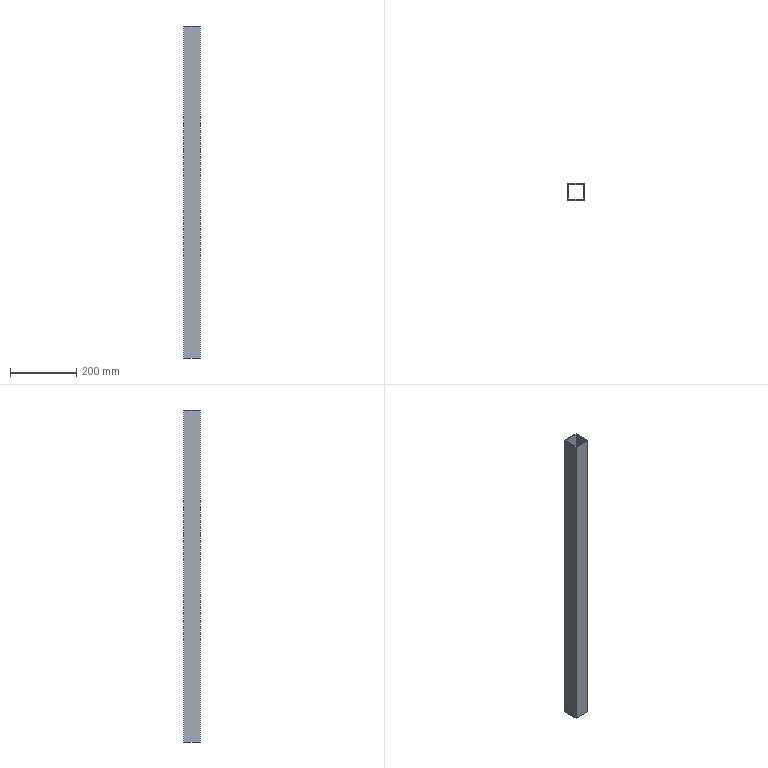Part | STEP file | BCC3 H19_5 | 1 solid | 10 faces | box 50 x 50 x 1000 mm | volume 564000 mm3 | plane 10
STEP:
#1=CARTESIAN_POINT('',(0.,0.,0.));
#2=DIRECTION('',(0.,0.,1.));
#3=DIRECTION('',(1.,0.,0.));
#4=AXIS2_PLACEMENT_3D('',#1,#2,#3);
#5=CARTESIAN_POINT('',(-25.,25.,500.));
#6=VERTEX_POINT('',#5);
#7=CARTESIAN_POINT('',(-25.,-25.,500.));
#8=VERTEX_POINT('',#7);
#9=CARTESIAN_POINT('',(-25.,25.,500.));
#10=DIRECTION('',(0.,-1.,0.));
#11=VECTOR('',#10,1.);
#12=LINE('',#9,#11);
#13=CARTESIAN_POINT('',(0.,0.,500.));
#14=DIRECTION('',(0.,0.,1.));
#15=DIRECTION('',(1.,0.,0.));
#16=AXIS2_PLACEMENT_3D('',#13,#14,#15);
#17=PLANE('',#16);
#18=CARTESIAN_POINT('',(-25.,25.));
#19=DIRECTION('',(0.,-1.));
#20=VECTOR('',#19,1.);
#21=LINE('',#18,#20);
#22=(GEOMETRIC_REPRESENTATION_CONTEXT(2)PARAMETRIC_REPRESENTATION_CONTEXT()REPRESENTATION_CONTEXT('',''));
#23=DEFINITIONAL_REPRESENTATION('',(#21),#22);
#24=PCURVE('',#17,#23);
#25=CARTESIAN_POINT('',(-25.,25.,500.));
#26=DIRECTION('',(1.,0.,0.));
#27=DIRECTION('',(0.,1.,0.));
#28=AXIS2_PLACEMENT_3D('',#25,#26,#27);
#29=PLANE('',#28);
#30=CARTESIAN_POINT('',(0.,0.));
#31=DIRECTION('',(-1.,0.));
#32=VECTOR('',#31,1.);
#33=LINE('',#30,#32);
#34=(GEOMETRIC_REPRESENTATION_CONTEXT(2)PARAMETRIC_REPRESENTATION_CONTEXT()REPRESENTATION_CONTEXT('',''));
#35=DEFINITIONAL_REPRESENTATION('',(#33),#34);
#36=PCURVE('',#29,#35);
#37=SURFACE_CURVE('',#12,(#24,#36),.PCURVE_S1.);
#38=EDGE_CURVE('',#6,#8,#37,.T.);
#39=ORIENTED_EDGE('',*,*,#38,.T.);
#40=CARTESIAN_POINT('',(25.,-25.,500.));
#41=VERTEX_POINT('',#40);
#42=CARTESIAN_POINT('',(-25.,-25.,500.));
#43=DIRECTION('',(1.,0.,0.));
#44=VECTOR('',#43,1.);
#45=LINE('',#42,#44);
#46=CARTESIAN_POINT('',(-25.,-25.));
#47=DIRECTION('',(1.,0.));
#48=VECTOR('',#47,1.);
#49=LINE('',#46,#48);
#50=(GEOMETRIC_REPRESENTATION_CONTEXT(2)PARAMETRIC_REPRESENTATION_CONTEXT()REPRESENTATION_CONTEXT('',''));
#51=DEFINITIONAL_REPRESENTATION('',(#49),#50);
#52=PCURVE('',#17,#51);
#53=CARTESIAN_POINT('',(-25.,-25.,500.));
#54=DIRECTION('',(0.,1.,0.));
#55=DIRECTION('',(0.,0.,1.));
#56=AXIS2_PLACEMENT_3D('',#53,#54,#55);
#57=PLANE('',#56);
#58=CARTESIAN_POINT('',(0.,0.));
#59=DIRECTION('',(0.,1.));
#60=VECTOR('',#59,1.);
#61=LINE('',#58,#60);
#62=(GEOMETRIC_REPRESENTATION_CONTEXT(2)PARAMETRIC_REPRESENTATION_CONTEXT()REPRESENTATION_CONTEXT('',''));
#63=DEFINITIONAL_REPRESENTATION('',(#61),#62);
#64=PCURVE('',#57,#63);
#65=SURFACE_CURVE('',#45,(#52,#64),.PCURVE_S1.);
#66=EDGE_CURVE('',#8,#41,#65,.T.);
#67=ORIENTED_EDGE('',*,*,#66,.T.);
#68=CARTESIAN_POINT('',(25.,25.,500.));
#69=VERTEX_POINT('',#68);
#70=CARTESIAN_POINT('',(25.,25.,500.));
#71=DIRECTION('',(0.,1.,0.));
#72=VECTOR('',#71,1.);
#73=LINE('',#70,#72);
#74=CARTESIAN_POINT('',(25.,25.));
#75=DIRECTION('',(0.,1.));
#76=VECTOR('',#75,1.);
#77=LINE('',#74,#76);
#78=(GEOMETRIC_REPRESENTATION_CONTEXT(2)PARAMETRIC_REPRESENTATION_CONTEXT()REPRESENTATION_CONTEXT('',''));
#79=DEFINITIONAL_REPRESENTATION('',(#77),#78);
#80=PCURVE('',#17,#79);
#81=CARTESIAN_POINT('',(25.,25.,500.));
#82=DIRECTION('',(-1.,0.,0.));
#83=DIRECTION('',(0.,-1.,0.));
#84=AXIS2_PLACEMENT_3D('',#81,#82,#83);
#85=PLANE('',#84);
#86=CARTESIAN_POINT('',(0.,0.));
#87=DIRECTION('',(-1.,0.));
#88=VECTOR('',#87,1.);
#89=LINE('',#86,#88);
#90=(GEOMETRIC_REPRESENTATION_CONTEXT(2)PARAMETRIC_REPRESENTATION_CONTEXT()REPRESENTATION_CONTEXT('',''));
#91=DEFINITIONAL_REPRESENTATION('',(#89),#90);
#92=PCURVE('',#85,#91);
#93=SURFACE_CURVE('',#73,(#80,#92),.PCURVE_S1.);
#94=EDGE_CURVE('',#41,#69,#93,.T.);
#95=ORIENTED_EDGE('',*,*,#94,.T.);
#96=CARTESIAN_POINT('',(-25.,25.,500.));
#97=DIRECTION('',(-1.,0.,0.));
#98=VECTOR('',#97,1.);
#99=LINE('',#96,#98);
#100=CARTESIAN_POINT('',(-25.,25.));
#101=DIRECTION('',(-1.,0.));
#102=VECTOR('',#101,1.);
#103=LINE('',#100,#102);
#104=(GEOMETRIC_REPRESENTATION_CONTEXT(2)PARAMETRIC_REPRESENTATION_CONTEXT()REPRESENTATION_CONTEXT('',''));
#105=DEFINITIONAL_REPRESENTATION('',(#103),#104);
#106=PCURVE('',#17,#105);
#107=CARTESIAN_POINT('',(-25.,25.,500.));
#108=DIRECTION('',(0.,-1.,0.));
#109=DIRECTION('',(0.,0.,-1.));
#110=AXIS2_PLACEMENT_3D('',#107,#108,#109);
#111=PLANE('',#110);
#112=CARTESIAN_POINT('',(0.,0.));
#113=DIRECTION('',(0.,-1.));
#114=VECTOR('',#113,1.);
#115=LINE('',#112,#114);
#116=(GEOMETRIC_REPRESENTATION_CONTEXT(2)PARAMETRIC_REPRESENTATION_CONTEXT()REPRESENTATION_CONTEXT('',''));
#117=DEFINITIONAL_REPRESENTATION('',(#115),#116);
#118=PCURVE('',#111,#117);
#119=SURFACE_CURVE('',#99,(#106,#118),.PCURVE_S1.);
#120=EDGE_CURVE('',#69,#6,#119,.T.);
#121=ORIENTED_EDGE('',*,*,#120,.T.);
#122=EDGE_LOOP('',(#39,#67,#95,#121));
#123=FACE_BOUND('',#122,.T.);
#124=CARTESIAN_POINT('',(-22.,-22.,500.));
#125=VERTEX_POINT('',#124);
#126=CARTESIAN_POINT('',(22.,-22.,500.));
#127=VERTEX_POINT('',#126);
#128=CARTESIAN_POINT('',(-22.,-22.,500.));
#129=DIRECTION('',(1.,0.,0.));
#130=VECTOR('',#129,1.);
#131=LINE('',#128,#130);
#132=CARTESIAN_POINT('',(-22.,-22.));
#133=DIRECTION('',(1.,0.));
#134=VECTOR('',#133,1.);
#135=LINE('',#132,#134);
#136=(GEOMETRIC_REPRESENTATION_CONTEXT(2)PARAMETRIC_REPRESENTATION_CONTEXT()REPRESENTATION_CONTEXT('',''));
#137=DEFINITIONAL_REPRESENTATION('',(#135),#136);
#138=PCURVE('',#17,#137);
#139=CARTESIAN_POINT('',(-22.,-22.,500.));
#140=DIRECTION('',(0.,1.,0.));
#141=DIRECTION('',(-1.,0.,0.));
#142=AXIS2_PLACEMENT_3D('',#139,#140,#141);
#143=PLANE('',#142);
#144=CARTESIAN_POINT('',(0.,0.));
#145=DIRECTION('',(-1.,0.));
#146=VECTOR('',#145,1.);
#147=LINE('',#144,#146);
#148=(GEOMETRIC_REPRESENTATION_CONTEXT(2)PARAMETRIC_REPRESENTATION_CONTEXT()REPRESENTATION_CONTEXT('',''));
#149=DEFINITIONAL_REPRESENTATION('',(#147),#148);
#150=PCURVE('',#143,#149);
#151=SURFACE_CURVE('',#131,(#138,#150),.PCURVE_S1.);
#152=EDGE_CURVE('',#125,#127,#151,.T.);
#153=ORIENTED_EDGE('',*,*,#152,.F.);
#154=CARTESIAN_POINT('',(-22.,22.,500.));
#155=VERTEX_POINT('',#154);
#156=CARTESIAN_POINT('',(-22.,22.,500.));
#157=DIRECTION('',(0.,-1.,0.));
#158=VECTOR('',#157,1.);
#159=LINE('',#156,#158);
#160=CARTESIAN_POINT('',(-22.,22.));
#161=DIRECTION('',(0.,-1.));
#162=VECTOR('',#161,1.);
#163=LINE('',#160,#162);
#164=(GEOMETRIC_REPRESENTATION_CONTEXT(2)PARAMETRIC_REPRESENTATION_CONTEXT()REPRESENTATION_CONTEXT('',''));
#165=DEFINITIONAL_REPRESENTATION('',(#163),#164);
#166=PCURVE('',#17,#165);
#167=CARTESIAN_POINT('',(-22.,22.,500.));
#168=DIRECTION('',(1.,0.,0.));
#169=DIRECTION('',(0.,1.,0.));
#170=AXIS2_PLACEMENT_3D('',#167,#168,#169);
#171=PLANE('',#170);
#172=CARTESIAN_POINT('',(0.,0.));
#173=DIRECTION('',(-1.,0.));
#174=VECTOR('',#173,1.);
#175=LINE('',#172,#174);
#176=(GEOMETRIC_REPRESENTATION_CONTEXT(2)PARAMETRIC_REPRESENTATION_CONTEXT()REPRESENTATION_CONTEXT('',''));
#177=DEFINITIONAL_REPRESENTATION('',(#175),#176);
#178=PCURVE('',#171,#177);
#179=SURFACE_CURVE('',#159,(#166,#178),.PCURVE_S1.);
#180=EDGE_CURVE('',#155,#125,#179,.T.);
#181=ORIENTED_EDGE('',*,*,#180,.F.);
#182=CARTESIAN_POINT('',(22.,22.,500.));
#183=VERTEX_POINT('',#182);
#184=CARTESIAN_POINT('',(-22.,22.,500.));
#185=DIRECTION('',(-1.,0.,0.));
#186=VECTOR('',#185,1.);
#187=LINE('',#184,#186);
#188=CARTESIAN_POINT('',(-22.,22.));
#189=DIRECTION('',(-1.,0.));
#190=VECTOR('',#189,1.);
#191=LINE('',#188,#190);
#192=(GEOMETRIC_REPRESENTATION_CONTEXT(2)PARAMETRIC_REPRESENTATION_CONTEXT()REPRESENTATION_CONTEXT('',''));
#193=DEFINITIONAL_REPRESENTATION('',(#191),#192);
#194=PCURVE('',#17,#193);
#195=CARTESIAN_POINT('',(-22.,22.,500.));
#196=DIRECTION('',(0.,-1.,0.));
#197=DIRECTION('',(0.,0.,-1.));
#198=AXIS2_PLACEMENT_3D('',#195,#196,#197);
#199=PLANE('',#198);
#200=CARTESIAN_POINT('',(0.,0.));
#201=DIRECTION('',(0.,-1.));
#202=VECTOR('',#201,1.);
#203=LINE('',#200,#202);
#204=(GEOMETRIC_REPRESENTATION_CONTEXT(2)PARAMETRIC_REPRESENTATION_CONTEXT()REPRESENTATION_CONTEXT('',''));
#205=DEFINITIONAL_REPRESENTATION('',(#203),#204);
#206=PCURVE('',#199,#205);
#207=SURFACE_CURVE('',#187,(#194,#206),.PCURVE_S1.);
#208=EDGE_CURVE('',#183,#155,#207,.T.);
#209=ORIENTED_EDGE('',*,*,#208,.F.);
#210=CARTESIAN_POINT('',(22.,22.,500.));
#211=DIRECTION('',(0.,1.,0.));
#212=VECTOR('',#211,1.);
#213=LINE('',#210,#212);
#214=CARTESIAN_POINT('',(22.,22.));
#215=DIRECTION('',(0.,1.));
#216=VECTOR('',#215,1.);
#217=LINE('',#214,#216);
#218=(GEOMETRIC_REPRESENTATION_CONTEXT(2)PARAMETRIC_REPRESENTATION_CONTEXT()REPRESENTATION_CONTEXT('',''));
#219=DEFINITIONAL_REPRESENTATION('',(#217),#218);
#220=PCURVE('',#17,#219);
#221=CARTESIAN_POINT('',(22.,22.,500.));
#222=DIRECTION('',(-1.,0.,0.));
#223=DIRECTION('',(0.,-1.,0.));
#224=AXIS2_PLACEMENT_3D('',#221,#222,#223);
#225=PLANE('',#224);
#226=CARTESIAN_POINT('',(0.,0.));
#227=DIRECTION('',(-1.,0.));
#228=VECTOR('',#227,1.);
#229=LINE('',#226,#228);
#230=(GEOMETRIC_REPRESENTATION_CONTEXT(2)PARAMETRIC_REPRESENTATION_CONTEXT()REPRESENTATION_CONTEXT('',''));
#231=DEFINITIONAL_REPRESENTATION('',(#229),#230);
#232=PCURVE('',#225,#231);
#233=SURFACE_CURVE('',#213,(#220,#232),.PCURVE_S1.);
#234=EDGE_CURVE('',#127,#183,#233,.T.);
#235=ORIENTED_EDGE('',*,*,#234,.F.);
#236=EDGE_LOOP('',(#153,#181,#209,#235));
#237=FACE_BOUND('',#236,.T.);
#238=ADVANCED_FACE('',(#123,#237),#17,.T.);
#239=CARTESIAN_POINT('',(-25.,25.,-500.));
#240=VERTEX_POINT('',#239);
#241=CARTESIAN_POINT('',(-25.,-25.,-500.));
#242=VERTEX_POINT('',#241);
#243=CARTESIAN_POINT('',(-25.,25.,-500.));
#244=DIRECTION('',(0.,-1.,0.));
#245=VECTOR('',#244,1.);
#246=LINE('',#243,#245);
#247=CARTESIAN_POINT('',(0.,0.,-500.));
#248=DIRECTION('',(0.,0.,1.));
#249=DIRECTION('',(1.,0.,0.));
#250=AXIS2_PLACEMENT_3D('',#247,#248,#249);
#251=PLANE('',#250);
#252=CARTESIAN_POINT('',(-25.,25.));
#253=DIRECTION('',(0.,-1.));
#254=VECTOR('',#253,1.);
#255=LINE('',#252,#254);
#256=(GEOMETRIC_REPRESENTATION_CONTEXT(2)PARAMETRIC_REPRESENTATION_CONTEXT()REPRESENTATION_CONTEXT('',''));
#257=DEFINITIONAL_REPRESENTATION('',(#255),#256);
#258=PCURVE('',#251,#257);
#259=CARTESIAN_POINT('',(0.,-1000.));
#260=DIRECTION('',(-1.,0.));
#261=VECTOR('',#260,1.);
#262=LINE('',#259,#261);
#263=(GEOMETRIC_REPRESENTATION_CONTEXT(2)PARAMETRIC_REPRESENTATION_CONTEXT()REPRESENTATION_CONTEXT('',''));
#264=DEFINITIONAL_REPRESENTATION('',(#262),#263);
#265=PCURVE('',#29,#264);
#266=SURFACE_CURVE('',#246,(#258,#265),.PCURVE_S1.);
#267=EDGE_CURVE('',#240,#242,#266,.T.);
#268=ORIENTED_EDGE('',*,*,#267,.F.);
#269=CARTESIAN_POINT('',(25.,25.,-500.));
#270=VERTEX_POINT('',#269);
#271=CARTESIAN_POINT('',(-25.,25.,-500.));
#272=DIRECTION('',(-1.,0.,0.));
#273=VECTOR('',#272,1.);
#274=LINE('',#271,#273);
#275=CARTESIAN_POINT('',(-25.,25.));
#276=DIRECTION('',(-1.,0.));
#277=VECTOR('',#276,1.);
#278=LINE('',#275,#277);
#279=(GEOMETRIC_REPRESENTATION_CONTEXT(2)PARAMETRIC_REPRESENTATION_CONTEXT()REPRESENTATION_CONTEXT('',''));
#280=DEFINITIONAL_REPRESENTATION('',(#278),#279);
#281=PCURVE('',#251,#280);
#282=CARTESIAN_POINT('',(1000.,0.));
#283=DIRECTION('',(0.,-1.));
#284=VECTOR('',#283,1.);
#285=LINE('',#282,#284);
#286=(GEOMETRIC_REPRESENTATION_CONTEXT(2)PARAMETRIC_REPRESENTATION_CONTEXT()REPRESENTATION_CONTEXT('',''));
#287=DEFINITIONAL_REPRESENTATION('',(#285),#286);
#288=PCURVE('',#111,#287);
#289=SURFACE_CURVE('',#274,(#281,#288),.PCURVE_S1.);
#290=EDGE_CURVE('',#270,#240,#289,.T.);
#291=ORIENTED_EDGE('',*,*,#290,.F.);
#292=CARTESIAN_POINT('',(25.,-25.,-500.));
#293=VERTEX_POINT('',#292);
#294=CARTESIAN_POINT('',(25.,25.,-500.));
#295=DIRECTION('',(0.,1.,0.));
#296=VECTOR('',#295,1.);
#297=LINE('',#294,#296);
#298=CARTESIAN_POINT('',(25.,25.));
#299=DIRECTION('',(0.,1.));
#300=VECTOR('',#299,1.);
#301=LINE('',#298,#300);
#302=(GEOMETRIC_REPRESENTATION_CONTEXT(2)PARAMETRIC_REPRESENTATION_CONTEXT()REPRESENTATION_CONTEXT('',''));
#303=DEFINITIONAL_REPRESENTATION('',(#301),#302);
#304=PCURVE('',#251,#303);
#305=CARTESIAN_POINT('',(0.,-1000.));
#306=DIRECTION('',(-1.,0.));
#307=VECTOR('',#306,1.);
#308=LINE('',#305,#307);
#309=(GEOMETRIC_REPRESENTATION_CONTEXT(2)PARAMETRIC_REPRESENTATION_CONTEXT()REPRESENTATION_CONTEXT('',''));
#310=DEFINITIONAL_REPRESENTATION('',(#308),#309);
#311=PCURVE('',#85,#310);
#312=SURFACE_CURVE('',#297,(#304,#311),.PCURVE_S1.);
#313=EDGE_CURVE('',#293,#270,#312,.T.);
#314=ORIENTED_EDGE('',*,*,#313,.F.);
#315=CARTESIAN_POINT('',(-25.,-25.,-500.));
#316=DIRECTION('',(1.,0.,0.));
#317=VECTOR('',#316,1.);
#318=LINE('',#315,#317);
#319=CARTESIAN_POINT('',(-25.,-25.));
#320=DIRECTION('',(1.,0.));
#321=VECTOR('',#320,1.);
#322=LINE('',#319,#321);
#323=(GEOMETRIC_REPRESENTATION_CONTEXT(2)PARAMETRIC_REPRESENTATION_CONTEXT()REPRESENTATION_CONTEXT('',''));
#324=DEFINITIONAL_REPRESENTATION('',(#322),#323);
#325=PCURVE('',#251,#324);
#326=CARTESIAN_POINT('',(-1000.,0.));
#327=DIRECTION('',(0.,1.));
#328=VECTOR('',#327,1.);
#329=LINE('',#326,#328);
#330=(GEOMETRIC_REPRESENTATION_CONTEXT(2)PARAMETRIC_REPRESENTATION_CONTEXT()REPRESENTATION_CONTEXT('',''));
#331=DEFINITIONAL_REPRESENTATION('',(#329),#330);
#332=PCURVE('',#57,#331);
#333=SURFACE_CURVE('',#318,(#325,#332),.PCURVE_S1.);
#334=EDGE_CURVE('',#242,#293,#333,.T.);
#335=ORIENTED_EDGE('',*,*,#334,.F.);
#336=EDGE_LOOP('',(#268,#291,#314,#335));
#337=FACE_BOUND('',#336,.T.);
#338=CARTESIAN_POINT('',(-22.,22.,-500.));
#339=VERTEX_POINT('',#338);
#340=CARTESIAN_POINT('',(-22.,-22.,-500.));
#341=VERTEX_POINT('',#340);
#342=CARTESIAN_POINT('',(-22.,22.,-500.));
#343=DIRECTION('',(0.,-1.,0.));
#344=VECTOR('',#343,1.);
#345=LINE('',#342,#344);
#346=CARTESIAN_POINT('',(-22.,22.));
#347=DIRECTION('',(0.,-1.));
#348=VECTOR('',#347,1.);
#349=LINE('',#346,#348);
#350=(GEOMETRIC_REPRESENTATION_CONTEXT(2)PARAMETRIC_REPRESENTATION_CONTEXT()REPRESENTATION_CONTEXT('',''));
#351=DEFINITIONAL_REPRESENTATION('',(#349),#350);
#352=PCURVE('',#251,#351);
#353=CARTESIAN_POINT('',(0.,-1000.));
#354=DIRECTION('',(-1.,0.));
#355=VECTOR('',#354,1.);
#356=LINE('',#353,#355);
#357=(GEOMETRIC_REPRESENTATION_CONTEXT(2)PARAMETRIC_REPRESENTATION_CONTEXT()REPRESENTATION_CONTEXT('',''));
#358=DEFINITIONAL_REPRESENTATION('',(#356),#357);
#359=PCURVE('',#171,#358);
#360=SURFACE_CURVE('',#345,(#352,#359),.PCURVE_S1.);
#361=EDGE_CURVE('',#339,#341,#360,.T.);
#362=ORIENTED_EDGE('',*,*,#361,.T.);
#363=CARTESIAN_POINT('',(22.,-22.,-500.));
#364=VERTEX_POINT('',#363);
#365=CARTESIAN_POINT('',(-22.,-22.,-500.));
#366=DIRECTION('',(1.,0.,0.));
#367=VECTOR('',#366,1.);
#368=LINE('',#365,#367);
#369=CARTESIAN_POINT('',(-22.,-22.));
#370=DIRECTION('',(1.,0.));
#371=VECTOR('',#370,1.);
#372=LINE('',#369,#371);
#373=(GEOMETRIC_REPRESENTATION_CONTEXT(2)PARAMETRIC_REPRESENTATION_CONTEXT()REPRESENTATION_CONTEXT('',''));
#374=DEFINITIONAL_REPRESENTATION('',(#372),#373);
#375=PCURVE('',#251,#374);
#376=CARTESIAN_POINT('',(0.,-1000.));
#377=DIRECTION('',(-1.,0.));
#378=VECTOR('',#377,1.);
#379=LINE('',#376,#378);
#380=(GEOMETRIC_REPRESENTATION_CONTEXT(2)PARAMETRIC_REPRESENTATION_CONTEXT()REPRESENTATION_CONTEXT('',''));
#381=DEFINITIONAL_REPRESENTATION('',(#379),#380);
#382=PCURVE('',#143,#381);
#383=SURFACE_CURVE('',#368,(#375,#382),.PCURVE_S1.);
#384=EDGE_CURVE('',#341,#364,#383,.T.);
#385=ORIENTED_EDGE('',*,*,#384,.T.);
#386=CARTESIAN_POINT('',(22.,22.,-500.));
#387=VERTEX_POINT('',#386);
#388=CARTESIAN_POINT('',(22.,22.,-500.));
#389=DIRECTION('',(0.,1.,0.));
#390=VECTOR('',#389,1.);
#391=LINE('',#388,#390);
#392=CARTESIAN_POINT('',(22.,22.));
#393=DIRECTION('',(0.,1.));
#394=VECTOR('',#393,1.);
#395=LINE('',#392,#394);
#396=(GEOMETRIC_REPRESENTATION_CONTEXT(2)PARAMETRIC_REPRESENTATION_CONTEXT()REPRESENTATION_CONTEXT('',''));
#397=DEFINITIONAL_REPRESENTATION('',(#395),#396);
#398=PCURVE('',#251,#397);
#399=CARTESIAN_POINT('',(0.,-1000.));
#400=DIRECTION('',(-1.,0.));
#401=VECTOR('',#400,1.);
#402=LINE('',#399,#401);
#403=(GEOMETRIC_REPRESENTATION_CONTEXT(2)PARAMETRIC_REPRESENTATION_CONTEXT()REPRESENTATION_CONTEXT('',''));
#404=DEFINITIONAL_REPRESENTATION('',(#402),#403);
#405=PCURVE('',#225,#404);
#406=SURFACE_CURVE('',#391,(#398,#405),.PCURVE_S1.);
#407=EDGE_CURVE('',#364,#387,#406,.T.);
#408=ORIENTED_EDGE('',*,*,#407,.T.);
#409=CARTESIAN_POINT('',(-22.,22.,-500.));
#410=DIRECTION('',(-1.,0.,0.));
#411=VECTOR('',#410,1.);
#412=LINE('',#409,#411);
#413=CARTESIAN_POINT('',(-22.,22.));
#414=DIRECTION('',(-1.,0.));
#415=VECTOR('',#414,1.);
#416=LINE('',#413,#415);
#417=(GEOMETRIC_REPRESENTATION_CONTEXT(2)PARAMETRIC_REPRESENTATION_CONTEXT()REPRESENTATION_CONTEXT('',''));
#418=DEFINITIONAL_REPRESENTATION('',(#416),#417);
#419=PCURVE('',#251,#418);
#420=CARTESIAN_POINT('',(1000.,0.));
#421=DIRECTION('',(0.,-1.));
#422=VECTOR('',#421,1.);
#423=LINE('',#420,#422);
#424=(GEOMETRIC_REPRESENTATION_CONTEXT(2)PARAMETRIC_REPRESENTATION_CONTEXT()REPRESENTATION_CONTEXT('',''));
#425=DEFINITIONAL_REPRESENTATION('',(#423),#424);
#426=PCURVE('',#199,#425);
#427=SURFACE_CURVE('',#412,(#419,#426),.PCURVE_S1.);
#428=EDGE_CURVE('',#387,#339,#427,.T.);
#429=ORIENTED_EDGE('',*,*,#428,.T.);
#430=EDGE_LOOP('',(#362,#385,#408,#429));
#431=FACE_BOUND('',#430,.T.);
#432=ADVANCED_FACE('',(#337,#431),#251,.F.);
#433=ORIENTED_EDGE('',*,*,#267,.T.);
#434=CARTESIAN_POINT('',(-25.,-25.,500.));
#435=DIRECTION('',(0.,0.,-1.));
#436=VECTOR('',#435,1.);
#437=LINE('',#434,#436);
#438=CARTESIAN_POINT('',(-50.,0.));
#439=DIRECTION('',(0.,-1.));
#440=VECTOR('',#439,1.);
#441=LINE('',#438,#440);
#442=(GEOMETRIC_REPRESENTATION_CONTEXT(2)PARAMETRIC_REPRESENTATION_CONTEXT()REPRESENTATION_CONTEXT('',''));
#443=DEFINITIONAL_REPRESENTATION('',(#441),#442);
#444=PCURVE('',#29,#443);
#445=CARTESIAN_POINT('',(0.,0.));
#446=DIRECTION('',(-1.,0.));
#447=VECTOR('',#446,1.);
#448=LINE('',#445,#447);
#449=(GEOMETRIC_REPRESENTATION_CONTEXT(2)PARAMETRIC_REPRESENTATION_CONTEXT()REPRESENTATION_CONTEXT('',''));
#450=DEFINITIONAL_REPRESENTATION('',(#448),#449);
#451=PCURVE('',#57,#450);
#452=SURFACE_CURVE('',#437,(#444,#451),.PCURVE_S1.);
#453=EDGE_CURVE('',#8,#242,#452,.T.);
#454=ORIENTED_EDGE('',*,*,#453,.F.);
#455=ORIENTED_EDGE('',*,*,#38,.F.);
#456=CARTESIAN_POINT('',(-25.,25.,500.));
#457=DIRECTION('',(0.,0.,-1.));
#458=VECTOR('',#457,1.);
#459=LINE('',#456,#458);
#460=CARTESIAN_POINT('',(0.,0.));
#461=DIRECTION('',(0.,-1.));
#462=VECTOR('',#461,1.);
#463=LINE('',#460,#462);
#464=(GEOMETRIC_REPRESENTATION_CONTEXT(2)PARAMETRIC_REPRESENTATION_CONTEXT()REPRESENTATION_CONTEXT('',''));
#465=DEFINITIONAL_REPRESENTATION('',(#463),#464);
#466=PCURVE('',#29,#465);
#467=CARTESIAN_POINT('',(0.,0.));
#468=DIRECTION('',(1.,0.));
#469=VECTOR('',#468,1.);
#470=LINE('',#467,#469);
#471=(GEOMETRIC_REPRESENTATION_CONTEXT(2)PARAMETRIC_REPRESENTATION_CONTEXT()REPRESENTATION_CONTEXT('',''));
#472=DEFINITIONAL_REPRESENTATION('',(#470),#471);
#473=PCURVE('',#111,#472);
#474=SURFACE_CURVE('',#459,(#466,#473),.PCURVE_S1.);
#475=EDGE_CURVE('',#6,#240,#474,.T.);
#476=ORIENTED_EDGE('',*,*,#475,.T.);
#477=EDGE_LOOP('',(#433,#454,#455,#476));
#478=FACE_BOUND('',#477,.T.);
#479=ADVANCED_FACE('',(#478),#29,.F.);
#480=ORIENTED_EDGE('',*,*,#334,.T.);
#481=CARTESIAN_POINT('',(25.,-25.,500.));
#482=DIRECTION('',(0.,0.,-1.));
#483=VECTOR('',#482,1.);
#484=LINE('',#481,#483);
#485=CARTESIAN_POINT('',(0.,50.));
#486=DIRECTION('',(-1.,0.));
#487=VECTOR('',#486,1.);
#488=LINE('',#485,#487);
#489=(GEOMETRIC_REPRESENTATION_CONTEXT(2)PARAMETRIC_REPRESENTATION_CONTEXT()REPRESENTATION_CONTEXT('',''));
#490=DEFINITIONAL_REPRESENTATION('',(#488),#489);
#491=PCURVE('',#57,#490);
#492=CARTESIAN_POINT('',(50.,0.));
#493=DIRECTION('',(0.,-1.));
#494=VECTOR('',#493,1.);
#495=LINE('',#492,#494);
#496=(GEOMETRIC_REPRESENTATION_CONTEXT(2)PARAMETRIC_REPRESENTATION_CONTEXT()REPRESENTATION_CONTEXT('',''));
#497=DEFINITIONAL_REPRESENTATION('',(#495),#496);
#498=PCURVE('',#85,#497);
#499=SURFACE_CURVE('',#484,(#491,#498),.PCURVE_S1.);
#500=EDGE_CURVE('',#41,#293,#499,.T.);
#501=ORIENTED_EDGE('',*,*,#500,.F.);
#502=ORIENTED_EDGE('',*,*,#66,.F.);
#503=ORIENTED_EDGE('',*,*,#453,.T.);
#504=EDGE_LOOP('',(#480,#501,#502,#503));
#505=FACE_BOUND('',#504,.T.);
#506=ADVANCED_FACE('',(#505),#57,.F.);
#507=ORIENTED_EDGE('',*,*,#313,.T.);
#508=CARTESIAN_POINT('',(25.,25.,500.));
#509=DIRECTION('',(0.,0.,-1.));
#510=VECTOR('',#509,1.);
#511=LINE('',#508,#510);
#512=CARTESIAN_POINT('',(0.,0.));
#513=DIRECTION('',(0.,-1.));
#514=VECTOR('',#513,1.);
#515=LINE('',#512,#514);
#516=(GEOMETRIC_REPRESENTATION_CONTEXT(2)PARAMETRIC_REPRESENTATION_CONTEXT()REPRESENTATION_CONTEXT('',''));
#517=DEFINITIONAL_REPRESENTATION('',(#515),#516);
#518=PCURVE('',#85,#517);
#519=CARTESIAN_POINT('',(0.,50.));
#520=DIRECTION('',(1.,0.));
#521=VECTOR('',#520,1.);
#522=LINE('',#519,#521);
#523=(GEOMETRIC_REPRESENTATION_CONTEXT(2)PARAMETRIC_REPRESENTATION_CONTEXT()REPRESENTATION_CONTEXT('',''));
#524=DEFINITIONAL_REPRESENTATION('',(#522),#523);
#525=PCURVE('',#111,#524);
#526=SURFACE_CURVE('',#511,(#518,#525),.PCURVE_S1.);
#527=EDGE_CURVE('',#69,#270,#526,.T.);
#528=ORIENTED_EDGE('',*,*,#527,.F.);
#529=ORIENTED_EDGE('',*,*,#94,.F.);
#530=ORIENTED_EDGE('',*,*,#500,.T.);
#531=EDGE_LOOP('',(#507,#528,#529,#530));
#532=FACE_BOUND('',#531,.T.);
#533=ADVANCED_FACE('',(#532),#85,.F.);
#534=ORIENTED_EDGE('',*,*,#290,.T.);
#535=ORIENTED_EDGE('',*,*,#475,.F.);
#536=ORIENTED_EDGE('',*,*,#120,.F.);
#537=ORIENTED_EDGE('',*,*,#527,.T.);
#538=EDGE_LOOP('',(#534,#535,#536,#537));
#539=FACE_BOUND('',#538,.T.);
#540=ADVANCED_FACE('',(#539),#111,.F.);
#541=ORIENTED_EDGE('',*,*,#361,.F.);
#542=CARTESIAN_POINT('',(-22.,22.,500.));
#543=DIRECTION('',(0.,0.,-1.));
#544=VECTOR('',#543,1.);
#545=LINE('',#542,#544);
#546=CARTESIAN_POINT('',(0.,0.));
#547=DIRECTION('',(0.,-1.));
#548=VECTOR('',#547,1.);
#549=LINE('',#546,#548);
#550=(GEOMETRIC_REPRESENTATION_CONTEXT(2)PARAMETRIC_REPRESENTATION_CONTEXT()REPRESENTATION_CONTEXT('',''));
#551=DEFINITIONAL_REPRESENTATION('',(#549),#550);
#552=PCURVE('',#171,#551);
#553=CARTESIAN_POINT('',(0.,0.));
#554=DIRECTION('',(1.,0.));
#555=VECTOR('',#554,1.);
#556=LINE('',#553,#555);
#557=(GEOMETRIC_REPRESENTATION_CONTEXT(2)PARAMETRIC_REPRESENTATION_CONTEXT()REPRESENTATION_CONTEXT('',''));
#558=DEFINITIONAL_REPRESENTATION('',(#556),#557);
#559=PCURVE('',#199,#558);
#560=SURFACE_CURVE('',#545,(#552,#559),.PCURVE_S1.);
#561=EDGE_CURVE('',#155,#339,#560,.T.);
#562=ORIENTED_EDGE('',*,*,#561,.F.);
#563=ORIENTED_EDGE('',*,*,#180,.T.);
#564=CARTESIAN_POINT('',(-22.,-22.,500.));
#565=DIRECTION('',(0.,0.,-1.));
#566=VECTOR('',#565,1.);
#567=LINE('',#564,#566);
#568=CARTESIAN_POINT('',(-44.,0.));
#569=DIRECTION('',(0.,-1.));
#570=VECTOR('',#569,1.);
#571=LINE('',#568,#570);
#572=(GEOMETRIC_REPRESENTATION_CONTEXT(2)PARAMETRIC_REPRESENTATION_CONTEXT()REPRESENTATION_CONTEXT('',''));
#573=DEFINITIONAL_REPRESENTATION('',(#571),#572);
#574=PCURVE('',#171,#573);
#575=CARTESIAN_POINT('',(0.,0.));
#576=DIRECTION('',(0.,-1.));
#577=VECTOR('',#576,1.);
#578=LINE('',#575,#577);
#579=(GEOMETRIC_REPRESENTATION_CONTEXT(2)PARAMETRIC_REPRESENTATION_CONTEXT()REPRESENTATION_CONTEXT('',''));
#580=DEFINITIONAL_REPRESENTATION('',(#578),#579);
#581=PCURVE('',#143,#580);
#582=SURFACE_CURVE('',#567,(#574,#581),.PCURVE_S1.);
#583=EDGE_CURVE('',#125,#341,#582,.T.);
#584=ORIENTED_EDGE('',*,*,#583,.T.);
#585=EDGE_LOOP('',(#541,#562,#563,#584));
#586=FACE_BOUND('',#585,.T.);
#587=ADVANCED_FACE('',(#586),#171,.T.);
#588=ORIENTED_EDGE('',*,*,#384,.F.);
#589=ORIENTED_EDGE('',*,*,#583,.F.);
#590=ORIENTED_EDGE('',*,*,#152,.T.);
#591=CARTESIAN_POINT('',(22.,-22.,500.));
#592=DIRECTION('',(0.,0.,-1.));
#593=VECTOR('',#592,1.);
#594=LINE('',#591,#593);
#595=CARTESIAN_POINT('',(-44.,0.));
#596=DIRECTION('',(0.,-1.));
#597=VECTOR('',#596,1.);
#598=LINE('',#595,#597);
#599=(GEOMETRIC_REPRESENTATION_CONTEXT(2)PARAMETRIC_REPRESENTATION_CONTEXT()REPRESENTATION_CONTEXT('',''));
#600=DEFINITIONAL_REPRESENTATION('',(#598),#599);
#601=PCURVE('',#143,#600);
#602=CARTESIAN_POINT('',(44.,0.));
#603=DIRECTION('',(0.,-1.));
#604=VECTOR('',#603,1.);
#605=LINE('',#602,#604);
#606=(GEOMETRIC_REPRESENTATION_CONTEXT(2)PARAMETRIC_REPRESENTATION_CONTEXT()REPRESENTATION_CONTEXT('',''));
#607=DEFINITIONAL_REPRESENTATION('',(#605),#606);
#608=PCURVE('',#225,#607);
#609=SURFACE_CURVE('',#594,(#601,#608),.PCURVE_S1.);
#610=EDGE_CURVE('',#127,#364,#609,.T.);
#611=ORIENTED_EDGE('',*,*,#610,.T.);
#612=EDGE_LOOP('',(#588,#589,#590,#611));
#613=FACE_BOUND('',#612,.T.);
#614=ADVANCED_FACE('',(#613),#143,.T.);
#615=ORIENTED_EDGE('',*,*,#407,.F.);
#616=ORIENTED_EDGE('',*,*,#610,.F.);
#617=ORIENTED_EDGE('',*,*,#234,.T.);
#618=CARTESIAN_POINT('',(22.,22.,500.));
#619=DIRECTION('',(0.,0.,-1.));
#620=VECTOR('',#619,1.);
#621=LINE('',#618,#620);
#622=CARTESIAN_POINT('',(0.,0.));
#623=DIRECTION('',(0.,-1.));
#624=VECTOR('',#623,1.);
#625=LINE('',#622,#624);
#626=(GEOMETRIC_REPRESENTATION_CONTEXT(2)PARAMETRIC_REPRESENTATION_CONTEXT()REPRESENTATION_CONTEXT('',''));
#627=DEFINITIONAL_REPRESENTATION('',(#625),#626);
#628=PCURVE('',#225,#627);
#629=CARTESIAN_POINT('',(0.,44.));
#630=DIRECTION('',(1.,0.));
#631=VECTOR('',#630,1.);
#632=LINE('',#629,#631);
#633=(GEOMETRIC_REPRESENTATION_CONTEXT(2)PARAMETRIC_REPRESENTATION_CONTEXT()REPRESENTATION_CONTEXT('',''));
#634=DEFINITIONAL_REPRESENTATION('',(#632),#633);
#635=PCURVE('',#199,#634);
#636=SURFACE_CURVE('',#621,(#628,#635),.PCURVE_S1.);
#637=EDGE_CURVE('',#183,#387,#636,.T.);
#638=ORIENTED_EDGE('',*,*,#637,.T.);
#639=EDGE_LOOP('',(#615,#616,#617,#638));
#640=FACE_BOUND('',#639,.T.);
#641=ADVANCED_FACE('',(#640),#225,.T.);
#642=ORIENTED_EDGE('',*,*,#428,.F.);
#643=ORIENTED_EDGE('',*,*,#637,.F.);
#644=ORIENTED_EDGE('',*,*,#208,.T.);
#645=ORIENTED_EDGE('',*,*,#561,.T.);
#646=EDGE_LOOP('',(#642,#643,#644,#645));
#647=FACE_BOUND('',#646,.T.);
#648=ADVANCED_FACE('',(#647),#199,.T.);
#649=CLOSED_SHELL('',(#238,#432,#479,#506,#533,#540,#587,#614,#641,#648));
#650=MANIFOLD_SOLID_BREP('',#649);
#651=(LENGTH_UNIT()NAMED_UNIT(*)SI_UNIT(.MILLI.,.METRE.));
#652=UNCERTAINTY_MEASURE_WITH_UNIT(LENGTH_MEASURE(0.0000001),#651,'','');
#653=(NAMED_UNIT(*)PLANE_ANGLE_UNIT()SI_UNIT($,.RADIAN.));
#654=(NAMED_UNIT(*)SI_UNIT($,.STERADIAN.)SOLID_ANGLE_UNIT());
#655=(GEOMETRIC_REPRESENTATION_CONTEXT(3)GLOBAL_UNCERTAINTY_ASSIGNED_CONTEXT((#652))GLOBAL_UNIT_ASSIGNED_CONTEXT((#651,#653,#654))REPRESENTATION_CONTEXT('',''));
#656=ADVANCED_BREP_SHAPE_REPRESENTATION('',(#4,#650),#655);